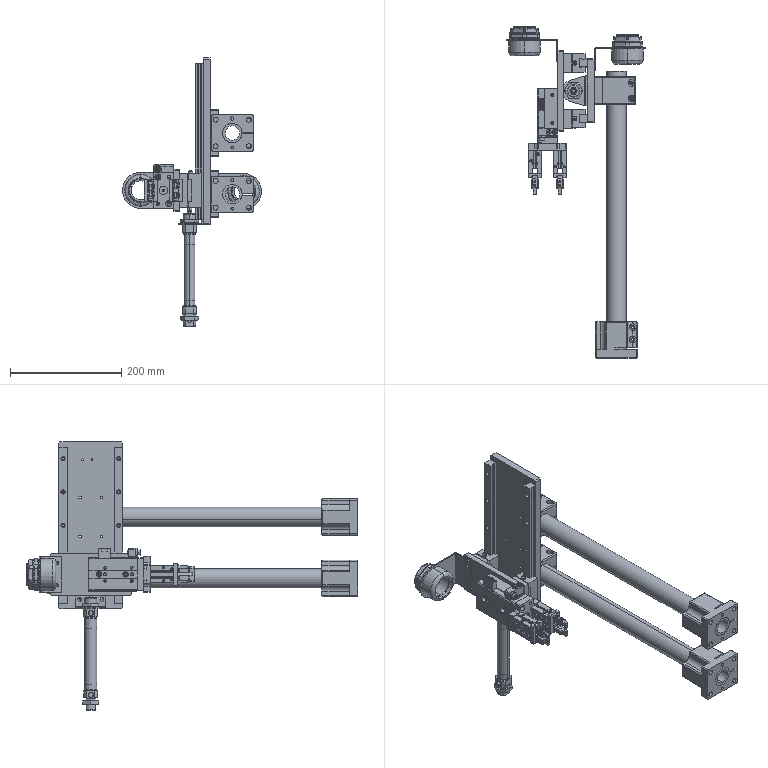Part | SolidWorks | 40 solids | 2314 faces | box 250 x 596.5 x 482 mm | volume 2400712 mm3 | plane 1012 | cylinder 912 | cone 344 | spline 38 | torus 8 | commonest cylinder face diameters 4 x87 5 x44 52 x44 9 x37 4.134 x36 4.5 x36